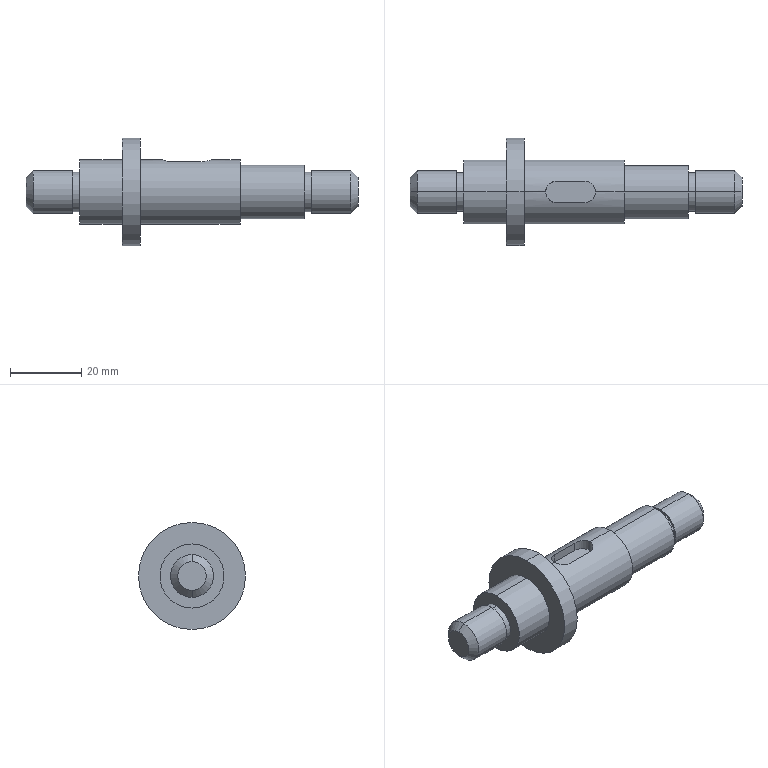Part | NX | features BREP 1 | 1 solid | 35 faces | box 93 x 30 x 30 mm | volume 19864 mm3 | cylinder 19 | plane 12 | cone 4 | commonest cylinder face diameters 11 x4 12 x4 18 x4 6 x3 15 x2 30 x2
STEP:
#1=CARTESIAN_POINT('',(11.521,0.,6.));
#2=VERTEX_POINT('',#1);
#3=CARTESIAN_POINT('',(8.521,3.,6.));
#4=VERTEX_POINT('',#3);
#5=CARTESIAN_POINT('',(8.521,0.,6.));
#6=DIRECTION('',(0.,0.,1.));
#7=DIRECTION('',(1.,0.,0.));
#8=AXIS2_PLACEMENT_3D('',#5,#6,#7);
#9=CIRCLE('',#8,3.);
#10=EDGE_CURVE('',#2,#4,#9,.T.);
#11=ORIENTED_EDGE('',*,*,#10,.F.);
#12=CARTESIAN_POINT('',(11.521,0.,9.));
#13=VERTEX_POINT('',#12);
#14=CARTESIAN_POINT('',(11.521,0.,6.));
#15=DIRECTION('',(0.,0.,1.));
#16=VECTOR('',#15,1000.);
#17=LINE('',#14,#16);
#18=EDGE_CURVE('',#2,#13,#17,.T.);
#19=ORIENTED_EDGE('',*,*,#18,.T.);
#20=CARTESIAN_POINT('',(8.521,3.,8.485));
#21=VERTEX_POINT('',#20);
#22=CARTESIAN_POINT('',(8.521,3.,8.485));
#23=CARTESIAN_POINT('',(9.32,3.,8.485));
#24=CARTESIAN_POINT('',(10.863,2.345,8.75));
#25=CARTESIAN_POINT('',(11.521,0.7985,9.));
#26=CARTESIAN_POINT('',(11.521,0.,9.));
#27=B_SPLINE_CURVE_WITH_KNOTS('',3,(#22,#23,#24,#25,#26),.UNSPECIFIED.,.F.,.F.,(4,1,4),(0.,0.00236,0.004721),.UNSPECIFIED.);
#28=EDGE_CURVE('',#21,#13,#27,.T.);
#29=ORIENTED_EDGE('',*,*,#28,.F.);
#30=CARTESIAN_POINT('',(8.521,3.,6.));
#31=DIRECTION('',(0.,0.,1.));
#32=VECTOR('',#31,1000.);
#33=LINE('',#30,#32);
#34=EDGE_CURVE('',#4,#21,#33,.T.);
#35=ORIENTED_EDGE('',*,*,#34,.F.);
#36=EDGE_LOOP('',(#11,#19,#29,#35));
#37=FACE_BOUND('',#36,.T.);
#38=CARTESIAN_POINT('',(8.521,0.,6.));
#39=DIRECTION('',(0.,0.,1.));
#40=DIRECTION('',(-1.,0.,0.));
#41=AXIS2_PLACEMENT_3D('',#38,#39,#40);
#42=CYLINDRICAL_SURFACE('',#41,3.);
#43=ADVANCED_FACE('',(#37),#42,.F.);
#44=CARTESIAN_POINT('',(52.521,0.,4.));
#45=VERTEX_POINT('',#44);
#46=CARTESIAN_POINT('',(52.521,0.,-4.));
#47=VERTEX_POINT('',#46);
#48=CARTESIAN_POINT('',(52.521,0.,0.));
#49=DIRECTION('',(-1.,0.,0.));
#50=DIRECTION('',(0.,0.,1.));
#51=AXIS2_PLACEMENT_3D('',#48,#49,#50);
#52=CIRCLE('',#51,4.);
#53=EDGE_CURVE('',#45,#47,#52,.T.);
#54=ORIENTED_EDGE('',*,*,#53,.T.);
#55=CARTESIAN_POINT('',(50.521,0.,-6.));
#56=VERTEX_POINT('',#55);
#57=CARTESIAN_POINT('',(52.521,0.,-4.));
#58=DIRECTION('',(-0.7071,0.,-0.7071));
#59=VECTOR('',#58,1000.);
#60=LINE('',#57,#59);
#61=EDGE_CURVE('',#47,#56,#60,.T.);
#62=ORIENTED_EDGE('',*,*,#61,.T.);
#63=CARTESIAN_POINT('',(50.521,0.,6.));
#64=VERTEX_POINT('',#63);
#65=CARTESIAN_POINT('',(50.521,0.,0.));
#66=DIRECTION('',(-1.,0.,0.));
#67=DIRECTION('',(0.,0.,1.));
#68=AXIS2_PLACEMENT_3D('',#65,#66,#67);
#69=CIRCLE('',#68,6.);
#70=EDGE_CURVE('',#64,#56,#69,.T.);
#71=ORIENTED_EDGE('',*,*,#70,.F.);
#72=CARTESIAN_POINT('',(52.521,0.,4.));
#73=DIRECTION('',(-0.7071,0.,0.7071));
#74=VECTOR('',#73,1000.);
#75=LINE('',#72,#74);
#76=EDGE_CURVE('',#45,#64,#75,.T.);
#77=ORIENTED_EDGE('',*,*,#76,.F.);
#78=EDGE_LOOP('',(#54,#62,#71,#77));
#79=FACE_BOUND('',#78,.T.);
#80=CARTESIAN_POINT('',(52.521,0.,0.));
#81=DIRECTION('',(-1.,0.,0.));
#82=DIRECTION('',(0.,0.,-1.));
#83=AXIS2_PLACEMENT_3D('',#80,#81,#82);
#84=CONICAL_SURFACE('',#83,4.,0.7854);
#85=ADVANCED_FACE('',(#79),#84,.T.);
#86=ORIENTED_EDGE('',*,*,#70,.T.);
#87=CARTESIAN_POINT('',(39.521,0.,-6.));
#88=VERTEX_POINT('',#87);
#89=CARTESIAN_POINT('',(-58.998,0.,-6.));
#90=DIRECTION('',(-1.,0.,0.));
#91=VECTOR('',#90,1000.);
#92=LINE('',#89,#91);
#93=EDGE_CURVE('',#56,#88,#92,.T.);
#94=ORIENTED_EDGE('',*,*,#93,.T.);
#95=CARTESIAN_POINT('',(39.521,0.,6.));
#96=VERTEX_POINT('',#95);
#97=CARTESIAN_POINT('',(39.521,0.,0.));
#98=DIRECTION('',(-1.,0.,0.));
#99=DIRECTION('',(0.,0.,1.));
#100=AXIS2_PLACEMENT_3D('',#97,#98,#99);
#101=CIRCLE('',#100,6.);
#102=EDGE_CURVE('',#96,#88,#101,.T.);
#103=ORIENTED_EDGE('',*,*,#102,.F.);
#104=CARTESIAN_POINT('',(-58.998,0.,6.));
#105=DIRECTION('',(-1.,0.,0.));
#106=VECTOR('',#105,1000.);
#107=LINE('',#104,#106);
#108=EDGE_CURVE('',#64,#96,#107,.T.);
#109=ORIENTED_EDGE('',*,*,#108,.F.);
#110=EDGE_LOOP('',(#86,#94,#103,#109));
#111=FACE_BOUND('',#110,.T.);
#112=CARTESIAN_POINT('',(-58.998,0.,0.));
#113=DIRECTION('',(-1.,0.,0.));
#114=DIRECTION('',(0.,0.,-1.));
#115=AXIS2_PLACEMENT_3D('',#112,#113,#114);
#116=CYLINDRICAL_SURFACE('',#115,6.);
#117=ADVANCED_FACE('',(#111),#116,.T.);
#118=CARTESIAN_POINT('',(39.521,0.,5.5));
#119=VERTEX_POINT('',#118);
#120=CARTESIAN_POINT('',(39.521,0.,-5.5));
#121=VERTEX_POINT('',#120);
#122=CARTESIAN_POINT('',(39.521,0.,0.));
#123=DIRECTION('',(-1.,0.,0.));
#124=DIRECTION('',(0.,0.,1.));
#125=AXIS2_PLACEMENT_3D('',#122,#123,#124);
#126=CIRCLE('',#125,5.5);
#127=EDGE_CURVE('',#119,#121,#126,.T.);
#128=ORIENTED_EDGE('',*,*,#127,.T.);
#129=CARTESIAN_POINT('',(37.521,0.,-5.5));
#130=VERTEX_POINT('',#129);
#131=CARTESIAN_POINT('',(-58.998,0.,-5.5));
#132=DIRECTION('',(-1.,0.,0.));
#133=VECTOR('',#132,1000.);
#134=LINE('',#131,#133);
#135=EDGE_CURVE('',#121,#130,#134,.T.);
#136=ORIENTED_EDGE('',*,*,#135,.T.);
#137=CARTESIAN_POINT('',(37.521,0.,5.5));
#138=VERTEX_POINT('',#137);
#139=CARTESIAN_POINT('',(37.521,0.,0.));
#140=DIRECTION('',(-1.,0.,0.));
#141=DIRECTION('',(0.,0.,1.));
#142=AXIS2_PLACEMENT_3D('',#139,#140,#141);
#143=CIRCLE('',#142,5.5);
#144=EDGE_CURVE('',#138,#130,#143,.T.);
#145=ORIENTED_EDGE('',*,*,#144,.F.);
#146=CARTESIAN_POINT('',(-58.998,0.,5.5));
#147=DIRECTION('',(-1.,0.,0.));
#148=VECTOR('',#147,1000.);
#149=LINE('',#146,#148);
#150=EDGE_CURVE('',#119,#138,#149,.T.);
#151=ORIENTED_EDGE('',*,*,#150,.F.);
#152=EDGE_LOOP('',(#128,#136,#145,#151));
#153=FACE_BOUND('',#152,.T.);
#154=CARTESIAN_POINT('',(-58.998,0.,0.));
#155=DIRECTION('',(-1.,0.,0.));
#156=DIRECTION('',(0.,0.,-1.));
#157=AXIS2_PLACEMENT_3D('',#154,#155,#156);
#158=CYLINDRICAL_SURFACE('',#157,5.5);
#159=ADVANCED_FACE('',(#153),#158,.T.);
#160=CARTESIAN_POINT('',(37.521,0.,7.5));
#161=VERTEX_POINT('',#160);
#162=CARTESIAN_POINT('',(37.521,0.,-7.5));
#163=VERTEX_POINT('',#162);
#164=CARTESIAN_POINT('',(37.521,0.,0.));
#165=DIRECTION('',(-1.,0.,0.));
#166=DIRECTION('',(0.,0.,1.));
#167=AXIS2_PLACEMENT_3D('',#164,#165,#166);
#168=CIRCLE('',#167,7.5);
#169=EDGE_CURVE('',#161,#163,#168,.T.);
#170=ORIENTED_EDGE('',*,*,#169,.T.);
#171=CARTESIAN_POINT('',(19.521,0.,-7.5));
#172=VERTEX_POINT('',#171);
#173=CARTESIAN_POINT('',(-58.998,0.,-7.5));
#174=DIRECTION('',(-1.,0.,0.));
#175=VECTOR('',#174,1000.);
#176=LINE('',#173,#175);
#177=EDGE_CURVE('',#163,#172,#176,.T.);
#178=ORIENTED_EDGE('',*,*,#177,.T.);
#179=CARTESIAN_POINT('',(19.521,0.,7.5));
#180=VERTEX_POINT('',#179);
#181=CARTESIAN_POINT('',(19.521,0.,0.));
#182=DIRECTION('',(-1.,0.,0.));
#183=DIRECTION('',(0.,0.,1.));
#184=AXIS2_PLACEMENT_3D('',#181,#182,#183);
#185=CIRCLE('',#184,7.5);
#186=EDGE_CURVE('',#180,#172,#185,.T.);
#187=ORIENTED_EDGE('',*,*,#186,.F.);
#188=CARTESIAN_POINT('',(-58.998,0.,7.5));
#189=DIRECTION('',(-1.,0.,0.));
#190=VECTOR('',#189,1000.);
#191=LINE('',#188,#190);
#192=EDGE_CURVE('',#161,#180,#191,.T.);
#193=ORIENTED_EDGE('',*,*,#192,.F.);
#194=EDGE_LOOP('',(#170,#178,#187,#193));
#195=FACE_BOUND('',#194,.T.);
#196=CARTESIAN_POINT('',(-58.998,0.,0.));
#197=DIRECTION('',(-1.,0.,0.));
#198=DIRECTION('',(0.,0.,-1.));
#199=AXIS2_PLACEMENT_3D('',#196,#197,#198);
#200=CYLINDRICAL_SURFACE('',#199,7.5);
#201=ADVANCED_FACE('',(#195),#200,.T.);
#202=CARTESIAN_POINT('',(19.521,0.,9.));
#203=VERTEX_POINT('',#202);
#204=CARTESIAN_POINT('',(19.521,0.,-9.));
#205=VERTEX_POINT('',#204);
#206=CARTESIAN_POINT('',(19.521,0.,0.));
#207=DIRECTION('',(-1.,0.,0.));
#208=DIRECTION('',(0.,0.,1.));
#209=AXIS2_PLACEMENT_3D('',#206,#207,#208);
#210=CIRCLE('',#209,9.);
#211=EDGE_CURVE('',#203,#205,#210,.T.);
#212=ORIENTED_EDGE('',*,*,#211,.T.);
#213=CARTESIAN_POINT('',(-8.479,0.,-9.));
#214=VERTEX_POINT('',#213);
#215=CARTESIAN_POINT('',(-58.998,0.,-9.));
#216=DIRECTION('',(-1.,0.,0.));
#217=VECTOR('',#216,1000.);
#218=LINE('',#215,#217);
#219=EDGE_CURVE('',#205,#214,#218,.T.);
#220=ORIENTED_EDGE('',*,*,#219,.T.);
#221=CARTESIAN_POINT('',(-8.479,0.,9.));
#222=VERTEX_POINT('',#221);
#223=CARTESIAN_POINT('',(-8.479,0.,0.));
#224=DIRECTION('',(-1.,0.,0.));
#225=DIRECTION('',(0.,0.,1.));
#226=AXIS2_PLACEMENT_3D('',#223,#224,#225);
#227=CIRCLE('',#226,9.);
#228=EDGE_CURVE('',#222,#214,#227,.T.);
#229=ORIENTED_EDGE('',*,*,#228,.F.);
#230=CARTESIAN_POINT('',(-2.479,0.,9.));
#231=VERTEX_POINT('',#230);
#232=CARTESIAN_POINT('',(-58.998,0.,9.));
#233=DIRECTION('',(-1.,0.,0.));
#234=VECTOR('',#233,1000.);
#235=LINE('',#232,#234);
#236=EDGE_CURVE('',#231,#222,#235,.T.);
#237=ORIENTED_EDGE('',*,*,#236,.F.);
#238=CARTESIAN_POINT('',(0.5211,3.,8.485));
#239=VERTEX_POINT('',#238);
#240=CARTESIAN_POINT('',(-2.479,0.,9.));
#241=CARTESIAN_POINT('',(-2.479,0.7985,9.));
#242=CARTESIAN_POINT('',(-1.822,2.343,8.75));
#243=CARTESIAN_POINT('',(-0.2774,3.,8.485));
#244=CARTESIAN_POINT('',(0.5211,3.,8.485));
#245=B_SPLINE_CURVE_WITH_KNOTS('',3,(#240,#241,#242,#243,#244),.UNSPECIFIED.,.F.,.F.,(4,1,4),(0.,0.00236,0.004721),.UNSPECIFIED.);
#246=EDGE_CURVE('',#231,#239,#245,.T.);
#247=ORIENTED_EDGE('',*,*,#246,.T.);
#248=CARTESIAN_POINT('',(-58.998,3.,8.485));
#249=DIRECTION('',(1.,0.,0.));
#250=VECTOR('',#249,1000.);
#251=LINE('',#248,#250);
#252=EDGE_CURVE('',#239,#21,#251,.T.);
#253=ORIENTED_EDGE('',*,*,#252,.T.);
#254=ORIENTED_EDGE('',*,*,#28,.T.);
#255=CARTESIAN_POINT('',(-58.998,0.,9.));
#256=DIRECTION('',(-1.,0.,0.));
#257=VECTOR('',#256,1000.);
#258=LINE('',#255,#257);
#259=EDGE_CURVE('',#203,#13,#258,.T.);
#260=ORIENTED_EDGE('',*,*,#259,.F.);
#261=EDGE_LOOP('',(#212,#220,#229,#237,#247,#253,#254,#260));
#262=FACE_BOUND('',#261,.T.);
#263=CARTESIAN_POINT('',(-58.998,0.,0.));
#264=DIRECTION('',(-1.,0.,0.));
#265=DIRECTION('',(0.,0.,-1.));
#266=AXIS2_PLACEMENT_3D('',#263,#264,#265);
#267=CYLINDRICAL_SURFACE('',#266,9.);
#268=ADVANCED_FACE('',(#262),#267,.T.);
#269=CARTESIAN_POINT('',(-8.479,0.,15.));
#270=VERTEX_POINT('',#269);
#271=CARTESIAN_POINT('',(-8.479,0.,-15.));
#272=VERTEX_POINT('',#271);
#273=CARTESIAN_POINT('',(-8.479,0.,0.));
#274=DIRECTION('',(-1.,0.,0.));
#275=DIRECTION('',(0.,0.,1.));
#276=AXIS2_PLACEMENT_3D('',#273,#274,#275);
#277=CIRCLE('',#276,15.);
#278=EDGE_CURVE('',#270,#272,#277,.T.);
#279=ORIENTED_EDGE('',*,*,#278,.T.);
#280=CARTESIAN_POINT('',(-13.479,0.,-15.));
#281=VERTEX_POINT('',#280);
#282=CARTESIAN_POINT('',(-58.998,0.,-15.));
#283=DIRECTION('',(-1.,0.,0.));
#284=VECTOR('',#283,1000.);
#285=LINE('',#282,#284);
#286=EDGE_CURVE('',#272,#281,#285,.T.);
#287=ORIENTED_EDGE('',*,*,#286,.T.);
#288=CARTESIAN_POINT('',(-13.479,0.,15.));
#289=VERTEX_POINT('',#288);
#290=CARTESIAN_POINT('',(-13.479,0.,0.));
#291=DIRECTION('',(-1.,0.,0.));
#292=DIRECTION('',(0.,0.,1.));
#293=AXIS2_PLACEMENT_3D('',#290,#291,#292);
#294=CIRCLE('',#293,15.);
#295=EDGE_CURVE('',#289,#281,#294,.T.);
#296=ORIENTED_EDGE('',*,*,#295,.F.);
#297=CARTESIAN_POINT('',(-58.998,0.,15.));
#298=DIRECTION('',(-1.,0.,0.));
#299=VECTOR('',#298,1000.);
#300=LINE('',#297,#299);
#301=EDGE_CURVE('',#270,#289,#300,.T.);
#302=ORIENTED_EDGE('',*,*,#301,.F.);
#303=EDGE_LOOP('',(#279,#287,#296,#302));
#304=FACE_BOUND('',#303,.T.);
#305=CARTESIAN_POINT('',(-58.998,0.,0.));
#306=DIRECTION('',(-1.,0.,0.));
#307=DIRECTION('',(0.,0.,-1.));
#308=AXIS2_PLACEMENT_3D('',#305,#306,#307);
#309=CYLINDRICAL_SURFACE('',#308,15.);
#310=ADVANCED_FACE('',(#304),#309,.T.);
#311=CARTESIAN_POINT('',(-13.479,0.,9.));
#312=VERTEX_POINT('',#311);
#313=CARTESIAN_POINT('',(-13.479,0.,-9.));
#314=VERTEX_POINT('',#313);
#315=CARTESIAN_POINT('',(-13.479,0.,0.));
#316=DIRECTION('',(-1.,0.,0.));
#317=DIRECTION('',(0.,0.,1.));
#318=AXIS2_PLACEMENT_3D('',#315,#316,#317);
#319=CIRCLE('',#318,9.);
#320=EDGE_CURVE('',#312,#314,#319,.T.);
#321=ORIENTED_EDGE('',*,*,#320,.T.);
#322=CARTESIAN_POINT('',(-25.479,0.,-9.));
#323=VERTEX_POINT('',#322);
#324=CARTESIAN_POINT('',(-58.998,0.,-9.));
#325=DIRECTION('',(-1.,0.,0.));
#326=VECTOR('',#325,1000.);
#327=LINE('',#324,#326);
#328=EDGE_CURVE('',#314,#323,#327,.T.);
#329=ORIENTED_EDGE('',*,*,#328,.T.);
#330=CARTESIAN_POINT('',(-25.479,0.,9.));
#331=VERTEX_POINT('',#330);
#332=CARTESIAN_POINT('',(-25.479,0.,0.));
#333=DIRECTION('',(-1.,0.,0.));
#334=DIRECTION('',(0.,0.,1.));
#335=AXIS2_PLACEMENT_3D('',#332,#333,#334);
#336=CIRCLE('',#335,9.);
#337=EDGE_CURVE('',#331,#323,#336,.T.);
#338=ORIENTED_EDGE('',*,*,#337,.F.);
#339=CARTESIAN_POINT('',(-58.998,0.,9.));
#340=DIRECTION('',(-1.,0.,0.));
#341=VECTOR('',#340,1000.);
#342=LINE('',#339,#341);
#343=EDGE_CURVE('',#312,#331,#342,.T.);
#344=ORIENTED_EDGE('',*,*,#343,.F.);
#345=EDGE_LOOP('',(#321,#329,#338,#344));
#346=FACE_BOUND('',#345,.T.);
#347=CARTESIAN_POINT('',(-58.998,0.,0.));
#348=DIRECTION('',(-1.,0.,0.));
#349=DIRECTION('',(0.,0.,-1.));
#350=AXIS2_PLACEMENT_3D('',#347,#348,#349);
#351=CYLINDRICAL_SURFACE('',#350,9.);
#352=ADVANCED_FACE('',(#346),#351,.T.);
#353=CARTESIAN_POINT('',(-25.479,0.,5.5));
#354=VERTEX_POINT('',#353);
#355=CARTESIAN_POINT('',(-25.479,0.,-5.5));
#356=VERTEX_POINT('',#355);
#357=CARTESIAN_POINT('',(-25.479,0.,0.));
#358=DIRECTION('',(-1.,0.,0.));
#359=DIRECTION('',(0.,0.,1.));
#360=AXIS2_PLACEMENT_3D('',#357,#358,#359);
#361=CIRCLE('',#360,5.5);
#362=EDGE_CURVE('',#354,#356,#361,.T.);
#363=ORIENTED_EDGE('',*,*,#362,.T.);
#364=CARTESIAN_POINT('',(-27.479,0.,-5.5));
#365=VERTEX_POINT('',#364);
#366=CARTESIAN_POINT('',(-58.998,0.,-5.5));
#367=DIRECTION('',(-1.,0.,0.));
#368=VECTOR('',#367,1000.);
#369=LINE('',#366,#368);
#370=EDGE_CURVE('',#356,#365,#369,.T.);
#371=ORIENTED_EDGE('',*,*,#370,.T.);
#372=CARTESIAN_POINT('',(-27.479,0.,5.5));
#373=VERTEX_POINT('',#372);
#374=CARTESIAN_POINT('',(-27.479,0.,0.));
#375=DIRECTION('',(-1.,0.,0.));
#376=DIRECTION('',(0.,0.,1.));
#377=AXIS2_PLACEMENT_3D('',#374,#375,#376);
#378=CIRCLE('',#377,5.5);
#379=EDGE_CURVE('',#373,#365,#378,.T.);
#380=ORIENTED_EDGE('',*,*,#379,.F.);
#381=CARTESIAN_POINT('',(-58.998,0.,5.5));
#382=DIRECTION('',(-1.,0.,0.));
#383=VECTOR('',#382,1000.);
#384=LINE('',#381,#383);
#385=EDGE_CURVE('',#354,#373,#384,.T.);
#386=ORIENTED_EDGE('',*,*,#385,.F.);
#387=EDGE_LOOP('',(#363,#371,#380,#386));
#388=FACE_BOUND('',#387,.T.);
#389=CARTESIAN_POINT('',(-58.998,0.,0.));
#390=DIRECTION('',(-1.,0.,0.));
#391=DIRECTION('',(0.,0.,-1.));
#392=AXIS2_PLACEMENT_3D('',#389,#390,#391);
#393=CYLINDRICAL_SURFACE('',#392,5.5);
#394=ADVANCED_FACE('',(#388),#393,.T.);
#395=CARTESIAN_POINT('',(-27.479,0.,6.));
#396=VERTEX_POINT('',#395);
#397=CARTESIAN_POINT('',(-27.479,0.,-6.));
#398=VERTEX_POINT('',#397);
#399=CARTESIAN_POINT('',(-27.479,0.,0.));
#400=DIRECTION('',(-1.,0.,0.));
#401=DIRECTION('',(0.,0.,1.));
#402=AXIS2_PLACEMENT_3D('',#399,#400,#401);
#403=CIRCLE('',#402,6.);
#404=EDGE_CURVE('',#396,#398,#403,.T.);
#405=ORIENTED_EDGE('',*,*,#404,.T.);
#406=CARTESIAN_POINT('',(-38.479,0.,-6.));
#407=VERTEX_POINT('',#406);
#408=CARTESIAN_POINT('',(-58.998,0.,-6.));
#409=DIRECTION('',(-1.,0.,0.));
#410=VECTOR('',#409,1000.);
#411=LINE('',#408,#410);
#412=EDGE_CURVE('',#398,#407,#411,.T.);
#413=ORIENTED_EDGE('',*,*,#412,.T.);
#414=CARTESIAN_POINT('',(-38.479,0.,6.));
#415=VERTEX_POINT('',#414);
#416=CARTESIAN_POINT('',(-38.479,0.,0.));
#417=DIRECTION('',(-1.,0.,0.));
#418=DIRECTION('',(0.,0.,1.));
#419=AXIS2_PLACEMENT_3D('',#416,#417,#418);
#420=CIRCLE('',#419,6.);
#421=EDGE_CURVE('',#415,#407,#420,.T.);
#422=ORIENTED_EDGE('',*,*,#421,.F.);
#423=CARTESIAN_POINT('',(-58.998,0.,6.));
#424=DIRECTION('',(-1.,0.,0.));
#425=VECTOR('',#424,1000.);
#426=LINE('',#423,#425);
#427=EDGE_CURVE('',#396,#415,#426,.T.);
#428=ORIENTED_EDGE('',*,*,#427,.F.);
#429=EDGE_LOOP('',(#405,#413,#422,#428));
#430=FACE_BOUND('',#429,.T.);
#431=CARTESIAN_POINT('',(-58.998,0.,0.));
#432=DIRECTION('',(-1.,0.,0.));
#433=DIRECTION('',(0.,0.,-1.));
#434=AXIS2_PLACEMENT_3D('',#431,#432,#433);
#435=CYLINDRICAL_SURFACE('',#434,6.);
#436=ADVANCED_FACE('',(#430),#435,.T.);
#437=CARTESIAN_POINT('',(-40.479,0.,4.));
#438=VERTEX_POINT('',#437);
#439=CARTESIAN_POINT('',(-40.479,0.,-4.));
#440=VERTEX_POINT('',#439);
#441=CARTESIAN_POINT('',(-40.479,0.,0.));
#442=DIRECTION('',(-1.,0.,0.));
#443=DIRECTION('',(0.,0.,1.));
#444=AXIS2_PLACEMENT_3D('',#441,#442,#443);
#445=CIRCLE('',#444,4.);
#446=EDGE_CURVE('',#438,#440,#445,.T.);
#447=ORIENTED_EDGE('',*,*,#446,.F.);
#448=CARTESIAN_POINT('',(-38.479,0.,6.));
#449=DIRECTION('',(0.7071,0.,0.7071));
#450=VECTOR('',#449,1000.);
#451=LINE('',#448,#450);
#452=EDGE_CURVE('',#415,#438,#451,.F.);
#453=ORIENTED_EDGE('',*,*,#452,.F.);
#454=ORIENTED_EDGE('',*,*,#421,.T.);
#455=CARTESIAN_POINT('',(-38.479,0.,-6.));
#456=DIRECTION('',(0.7071,0.,-0.7071));
#457=VECTOR('',#456,1000.);
#458=LINE('',#455,#457);
#459=EDGE_CURVE('',#407,#440,#458,.F.);
#460=ORIENTED_EDGE('',*,*,#459,.T.);
#461=EDGE_LOOP('',(#447,#453,#454,#460));
#462=FACE_BOUND('',#461,.T.);
#463=CARTESIAN_POINT('',(-38.479,0.,0.));
#464=DIRECTION('',(1.,0.,0.));
#465=DIRECTION('',(0.,0.,1.));
#466=AXIS2_PLACEMENT_3D('',#463,#464,#465);
#467=CONICAL_SURFACE('',#466,6.,0.7854);
#468=ADVANCED_FACE('',(#462),#467,.T.);
#469=CARTESIAN_POINT('',(-40.479,0.,0.));
#470=DIRECTION('',(-1.,0.,0.));
#471=DIRECTION('',(0.,0.,1.));
#472=AXIS2_PLACEMENT_3D('',#469,#470,#471);
#473=CIRCLE('',#472,4.);
#474=EDGE_CURVE('',#440,#438,#473,.T.);
#475=ORIENTED_EDGE('',*,*,#474,.T.);
#476=ORIENTED_EDGE('',*,*,#446,.T.);
#477=EDGE_LOOP('',(#475,#476));
#478=FACE_BOUND('',#477,.T.);
#479=CARTESIAN_POINT('',(-40.479,0.,0.));
#480=DIRECTION('',(1.,0.,0.));
#481=DIRECTION('',(0.,1.,0.));
#482=AXIS2_PLACEMENT_3D('',#479,#480,#481);
#483=PLANE('',#482);
#484=ADVANCED_FACE('',(#478),#483,.F.);
#485=ORIENTED_EDGE('',*,*,#452,.T.);
#486=ORIENTED_EDGE('',*,*,#474,.F.);
#487=ORIENTED_EDGE('',*,*,#459,.F.);
#488=CARTESIAN_POINT('',(-38.479,0.,0.));
#489=DIRECTION('',(-1.,0.,0.));
#490=DIRECTION('',(0.,0.,1.));
#491=AXIS2_PLACEMENT_3D('',#488,#489,#490);
#492=CIRCLE('',#491,6.);
#493=EDGE_CURVE('',#407,#415,#492,.T.);
#494=ORIENTED_EDGE('',*,*,#493,.T.);
#495=EDGE_LOOP('',(#485,#486,#487,#494));
#496=FACE_BOUND('',#495,.T.);
#497=CARTESIAN_POINT('',(-38.479,0.,0.));
#498=DIRECTION('',(1.,0.,0.));
#499=DIRECTION('',(0.,0.,1.));
#500=AXIS2_PLACEMENT_3D('',#497,#498,#499);
#501=CONICAL_SURFACE('',#500,6.,0.7854);
#502=ADVANCED_FACE('',(#496),#501,.T.);
#503=ORIENTED_EDGE('',*,*,#412,.F.);
#504=CARTESIAN_POINT('',(-27.479,0.,0.));
#505=DIRECTION('',(-1.,0.,0.));
#506=DIRECTION('',(0.,0.,1.));
#507=AXIS2_PLACEMENT_3D('',#504,#505,#506);
#508=CIRCLE('',#507,6.);
#509=EDGE_CURVE('',#398,#396,#508,.T.);
#510=ORIENTED_EDGE('',*,*,#509,.T.);
#511=ORIENTED_EDGE('',*,*,#427,.T.);
#512=ORIENTED_EDGE('',*,*,#493,.F.);
#513=EDGE_LOOP('',(#503,#510,#511,#512));
#514=FACE_BOUND('',#513,.T.);
#515=CARTESIAN_POINT('',(-58.998,0.,0.));
#516=DIRECTION('',(-1.,0.,0.));
#517=DIRECTION('',(0.,0.,-1.));
#518=AXIS2_PLACEMENT_3D('',#515,#516,#517);
#519=CYLINDRICAL_SURFACE('',#518,6.);
#520=ADVANCED_FACE('',(#514),#519,.T.);
#521=ORIENTED_EDGE('',*,*,#404,.F.);
#522=ORIENTED_EDGE('',*,*,#509,.F.);
#523=EDGE_LOOP('',(#521,#522));
#524=FACE_BOUND('',#523,.T.);
#525=ORIENTED_EDGE('',*,*,#379,.T.);
#526=CARTESIAN_POINT('',(-27.479,0.,0.));
#527=DIRECTION('',(-1.,0.,0.));
#528=DIRECTION('',(0.,0.,1.));
#529=AXIS2_PLACEMENT_3D('',#526,#527,#528);
#530=CIRCLE('',#529,5.5);
#531=EDGE_CURVE('',#365,#373,#530,.T.);
#532=ORIENTED_EDGE('',*,*,#531,.T.);
#533=EDGE_LOOP('',(#525,#532));
#534=FACE_BOUND('',#533,.T.);
#535=CARTESIAN_POINT('',(-27.479,6.,0.));
#536=DIRECTION('',(-1.,0.,0.));
#537=DIRECTION('',(0.,0.,-1.));
#538=AXIS2_PLACEMENT_3D('',#535,#536,#537);
#539=PLANE('',#538);
#540=ADVANCED_FACE('',(#524,#534),#539,.F.);
#541=ORIENTED_EDGE('',*,*,#370,.F.);
#542=CARTESIAN_POINT('',(-25.479,0.,0.));
#543=DIRECTION('',(-1.,0.,0.));
#544=DIRECTION('',(0.,0.,1.));
#545=AXIS2_PLACEMENT_3D('',#542,#543,#544);
#546=CIRCLE('',#545,5.5);
#547=EDGE_CURVE('',#356,#354,#546,.T.);
#548=ORIENTED_EDGE('',*,*,#547,.T.);
#549=ORIENTED_EDGE('',*,*,#385,.T.);
#550=ORIENTED_EDGE('',*,*,#531,.F.);
#551=EDGE_LOOP('',(#541,#548,#549,#550));
#552=FACE_BOUND('',#551,.T.);
#553=CARTESIAN_POINT('',(-58.998,0.,0.));
#554=DIRECTION('',(-1.,0.,0.));
#555=DIRECTION('',(0.,0.,-1.));
#556=AXIS2_PLACEMENT_3D('',#553,#554,#555);
#557=CYLINDRICAL_SURFACE('',#556,5.5);
#558=ADVANCED_FACE('',(#552),#557,.T.);
#559=ORIENTED_EDGE('',*,*,#337,.T.);
#560=CARTESIAN_POINT('',(-25.479,0.,0.));
#561=DIRECTION('',(-1.,0.,0.));
#562=DIRECTION('',(0.,0.,1.));
#563=AXIS2_PLACEMENT_3D('',#560,#561,#562);
#564=CIRCLE('',#563,9.);
#565=EDGE_CURVE('',#323,#331,#564,.T.);
#566=ORIENTED_EDGE('',*,*,#565,.T.);
#567=EDGE_LOOP('',(#559,#566));
#568=FACE_BOUND('',#567,.T.);
#569=ORIENTED_EDGE('',*,*,#362,.F.);
#570=ORIENTED_EDGE('',*,*,#547,.F.);
#571=EDGE_LOOP('',(#569,#570));
#572=FACE_BOUND('',#571,.T.);
#573=CARTESIAN_POINT('',(-25.479,5.5,0.));
#574=DIRECTION('',(1.,0.,0.));
#575=DIRECTION('',(0.,1.,0.));
#576=AXIS2_PLACEMENT_3D('',#573,#574,#575);
#577=PLANE('',#576);
#578=ADVANCED_FACE('',(#568,#572),#577,.F.);
#579=ORIENTED_EDGE('',*,*,#328,.F.);
#580=CARTESIAN_POINT('',(-13.479,0.,0.));
#581=DIRECTION('',(-1.,0.,0.));
#582=DIRECTION('',(0.,0.,1.));
#583=AXIS2_PLACEMENT_3D('',#580,#581,#582);
#584=CIRCLE('',#583,9.);
#585=EDGE_CURVE('',#314,#312,#584,.T.);
#586=ORIENTED_EDGE('',*,*,#585,.T.);
#587=ORIENTED_EDGE('',*,*,#343,.T.);
#588=ORIENTED_EDGE('',*,*,#565,.F.);
#589=EDGE_LOOP('',(#579,#586,#587,#588));
#590=FACE_BOUND('',#589,.T.);
#591=CARTESIAN_POINT('',(-58.998,0.,0.));
#592=DIRECTION('',(-1.,0.,0.));
#593=DIRECTION('',(0.,0.,-1.));
#594=AXIS2_PLACEMENT_3D('',#591,#592,#593);
#595=CYLINDRICAL_SURFACE('',#594,9.);
#596=ADVANCED_FACE('',(#590),#595,.T.);
#597=ORIENTED_EDGE('',*,*,#295,.T.);
#598=CARTESIAN_POINT('',(-13.479,0.,0.));
#599=DIRECTION('',(-1.,0.,0.));
#600=DIRECTION('',(0.,0.,1.));
#601=AXIS2_PLACEMENT_3D('',#598,#599,#600);
#602=CIRCLE('',#601,15.);
#603=EDGE_CURVE('',#281,#289,#602,.T.);
#604=ORIENTED_EDGE('',*,*,#603,.T.);
#605=EDGE_LOOP('',(#597,#604));
#606=FACE_BOUND('',#605,.T.);
#607=ORIENTED_EDGE('',*,*,#320,.F.);
#608=ORIENTED_EDGE('',*,*,#585,.F.);
#609=EDGE_LOOP('',(#607,#608));
#610=FACE_BOUND('',#609,.T.);
#611=CARTESIAN_POINT('',(-13.479,9.,0.));
#612=DIRECTION('',(1.,0.,0.));
#613=DIRECTION('',(0.,1.,0.));
#614=AXIS2_PLACEMENT_3D('',#611,#612,#613);
#615=PLANE('',#614);
#616=ADVANCED_FACE('',(#606,#610),#615,.F.);
#617=ORIENTED_EDGE('',*,*,#286,.F.);
#618=CARTESIAN_POINT('',(-8.479,0.,0.));
#619=DIRECTION('',(-1.,0.,0.));
#620=DIRECTION('',(0.,0.,1.));
#621=AXIS2_PLACEMENT_3D('',#618,#619,#620);
#622=CIRCLE('',#621,15.);
#623=EDGE_CURVE('',#272,#270,#622,.T.);
#624=ORIENTED_EDGE('',*,*,#623,.T.);
#625=ORIENTED_EDGE('',*,*,#301,.T.);
#626=ORIENTED_EDGE('',*,*,#603,.F.);
#627=EDGE_LOOP('',(#617,#624,#625,#626));
#628=FACE_BOUND('',#627,.T.);
#629=CARTESIAN_POINT('',(-58.998,0.,0.));
#630=DIRECTION('',(-1.,0.,0.));
#631=DIRECTION('',(0.,0.,-1.));
#632=AXIS2_PLACEMENT_3D('',#629,#630,#631);
#633=CYLINDRICAL_SURFACE('',#632,15.);
#634=ADVANCED_FACE('',(#628),#633,.T.);
#635=ORIENTED_EDGE('',*,*,#278,.F.);
#636=ORIENTED_EDGE('',*,*,#623,.F.);
#637=EDGE_LOOP('',(#635,#636));
#638=FACE_BOUND('',#637,.T.);
#639=ORIENTED_EDGE('',*,*,#228,.T.);
#640=CARTESIAN_POINT('',(-8.479,0.,0.));
#641=DIRECTION('',(-1.,0.,0.));
#642=DIRECTION('',(0.,0.,1.));
#643=AXIS2_PLACEMENT_3D('',#640,#641,#642);
#644=CIRCLE('',#643,9.);
#645=EDGE_CURVE('',#214,#222,#644,.T.);
#646=ORIENTED_EDGE('',*,*,#645,.T.);
#647=EDGE_LOOP('',(#639,#646));
#648=FACE_BOUND('',#647,.T.);
#649=CARTESIAN_POINT('',(-8.479,15.,0.));
#650=DIRECTION('',(-1.,0.,0.));
#651=DIRECTION('',(0.,0.,-1.));
#652=AXIS2_PLACEMENT_3D('',#649,#650,#651);
#653=PLANE('',#652);
#654=ADVANCED_FACE('',(#638,#648),#653,.F.);
#655=ORIENTED_EDGE('',*,*,#219,.F.);
#656=CARTESIAN_POINT('',(19.521,0.,0.));
#657=DIRECTION('',(-1.,0.,0.));
#658=DIRECTION('',(0.,0.,1.));
#659=AXIS2_PLACEMENT_3D('',#656,#657,#658);
#660=CIRCLE('',#659,9.);
#661=EDGE_CURVE('',#205,#203,#660,.T.);
#662=ORIENTED_EDGE('',*,*,#661,.T.);
#663=ORIENTED_EDGE('',*,*,#259,.T.);
#664=CARTESIAN_POINT('',(8.521,-3.,8.485));
#665=VERTEX_POINT('',#664);
#666=CARTESIAN_POINT('',(11.521,0.,9.));
#667=CARTESIAN_POINT('',(11.521,-0.7985,9.));
#668=CARTESIAN_POINT('',(10.865,-2.343,8.75));
#669=CARTESIAN_POINT('',(9.32,-3.,8.485));
#670=CARTESIAN_POINT('',(8.521,-3.,8.485));
#671=B_SPLINE_CURVE_WITH_KNOTS('',3,(#666,#667,#668,#669,#670),.UNSPECIFIED.,.F.,.F.,(4,1,4),(0.,0.00236,0.004721),.UNSPECIFIED.);
#672=EDGE_CURVE('',#13,#665,#671,.T.);
#673=ORIENTED_EDGE('',*,*,#672,.T.);
#674=CARTESIAN_POINT('',(0.5211,-3.,8.485));
#675=VERTEX_POINT('',#674);
#676=CARTESIAN_POINT('',(-58.998,-3.,8.485));
#677=DIRECTION('',(-1.,0.,0.));
#678=VECTOR('',#677,1000.);
#679=LINE('',#676,#678);
#680=EDGE_CURVE('',#665,#675,#679,.T.);
#681=ORIENTED_EDGE('',*,*,#680,.T.);
#682=CARTESIAN_POINT('',(0.5211,-3.,8.485));
#683=CARTESIAN_POINT('',(-0.2774,-3.,8.485));
#684=CARTESIAN_POINT('',(-1.821,-2.345,8.75));
#685=CARTESIAN_POINT('',(-2.479,-0.7985,9.));
#686=CARTESIAN_POINT('',(-2.479,0.,9.));
#687=B_SPLINE_CURVE_WITH_KNOTS('',3,(#682,#683,#684,#685,#686),.UNSPECIFIED.,.F.,.F.,(4,1,4),(0.,0.00236,0.004721),.UNSPECIFIED.);
#688=EDGE_CURVE('',#675,#231,#687,.T.);
#689=ORIENTED_EDGE('',*,*,#688,.T.);
#690=ORIENTED_EDGE('',*,*,#236,.T.);
#691=ORIENTED_EDGE('',*,*,#645,.F.);
#692=EDGE_LOOP('',(#655,#662,#663,#673,#681,#689,#690,#691));
#693=FACE_BOUND('',#692,.T.);
#694=CARTESIAN_POINT('',(-58.998,0.,0.));
#695=DIRECTION('',(-1.,0.,0.));
#696=DIRECTION('',(0.,0.,-1.));
#697=AXIS2_PLACEMENT_3D('',#694,#695,#696);
#698=CYLINDRICAL_SURFACE('',#697,9.);
#699=ADVANCED_FACE('',(#693),#698,.T.);
#700=ORIENTED_EDGE('',*,*,#211,.F.);
#701=ORIENTED_EDGE('',*,*,#661,.F.);
#702=EDGE_LOOP('',(#700,#701));
#703=FACE_BOUND('',#702,.T.);
#704=ORIENTED_EDGE('',*,*,#186,.T.);
#705=CARTESIAN_POINT('',(19.521,0.,0.));
#706=DIRECTION('',(-1.,0.,0.));
#707=DIRECTION('',(0.,0.,1.));
#708=AXIS2_PLACEMENT_3D('',#705,#706,#707);
#709=CIRCLE('',#708,7.5);
#710=EDGE_CURVE('',#172,#180,#709,.T.);
#711=ORIENTED_EDGE('',*,*,#710,.T.);
#712=EDGE_LOOP('',(#704,#711));
#713=FACE_BOUND('',#712,.T.);
#714=CARTESIAN_POINT('',(19.521,9.,0.));
#715=DIRECTION('',(-1.,0.,0.));
#716=DIRECTION('',(0.,0.,-1.));
#717=AXIS2_PLACEMENT_3D('',#714,#715,#716);
#718=PLANE('',#717);
#719=ADVANCED_FACE('',(#703,#713),#718,.F.);
#720=ORIENTED_EDGE('',*,*,#177,.F.);
#721=CARTESIAN_POINT('',(37.521,0.,0.));
#722=DIRECTION('',(-1.,0.,0.));
#723=DIRECTION('',(0.,0.,1.));
#724=AXIS2_PLACEMENT_3D('',#721,#722,#723);
#725=CIRCLE('',#724,7.5);
#726=EDGE_CURVE('',#163,#161,#725,.T.);
#727=ORIENTED_EDGE('',*,*,#726,.T.);
#728=ORIENTED_EDGE('',*,*,#192,.T.);
#729=ORIENTED_EDGE('',*,*,#710,.F.);
#730=EDGE_LOOP('',(#720,#727,#728,#729));
#731=FACE_BOUND('',#730,.T.);
#732=CARTESIAN_POINT('',(-58.998,0.,0.));
#733=DIRECTION('',(-1.,0.,0.));
#734=DIRECTION('',(0.,0.,-1.));
#735=AXIS2_PLACEMENT_3D('',#732,#733,#734);
#736=CYLINDRICAL_SURFACE('',#735,7.5);
#737=ADVANCED_FACE('',(#731),#736,.T.);
#738=ORIENTED_EDGE('',*,*,#169,.F.);
#739=ORIENTED_EDGE('',*,*,#726,.F.);
#740=EDGE_LOOP('',(#738,#739));
#741=FACE_BOUND('',#740,.T.);
#742=ORIENTED_EDGE('',*,*,#144,.T.);
#743=CARTESIAN_POINT('',(37.521,0.,0.));
#744=DIRECTION('',(-1.,0.,0.));
#745=DIRECTION('',(0.,0.,1.));
#746=AXIS2_PLACEMENT_3D('',#743,#744,#745);
#747=CIRCLE('',#746,5.5);
#748=EDGE_CURVE('',#130,#138,#747,.T.);
#749=ORIENTED_EDGE('',*,*,#748,.T.);
#750=EDGE_LOOP('',(#742,#749));
#751=FACE_BOUND('',#750,.T.);
#752=CARTESIAN_POINT('',(37.521,7.5,0.));
#753=DIRECTION('',(-1.,0.,0.));
#754=DIRECTION('',(0.,0.,-1.));
#755=AXIS2_PLACEMENT_3D('',#752,#753,#754);
#756=PLANE('',#755);
#757=ADVANCED_FACE('',(#741,#751),#756,.F.);
#758=ORIENTED_EDGE('',*,*,#135,.F.);
#759=CARTESIAN_POINT('',(39.521,0.,0.));
#760=DIRECTION('',(-1.,0.,0.));
#761=DIRECTION('',(0.,0.,1.));
#762=AXIS2_PLACEMENT_3D('',#759,#760,#761);
#763=CIRCLE('',#762,5.5);
#764=EDGE_CURVE('',#121,#119,#763,.T.);
#765=ORIENTED_EDGE('',*,*,#764,.T.);
#766=ORIENTED_EDGE('',*,*,#150,.T.);
#767=ORIENTED_EDGE('',*,*,#748,.F.);
#768=EDGE_LOOP('',(#758,#765,#766,#767));
#769=FACE_BOUND('',#768,.T.);
#770=CARTESIAN_POINT('',(-58.998,0.,0.));
#771=DIRECTION('',(-1.,0.,0.));
#772=DIRECTION('',(0.,0.,-1.));
#773=AXIS2_PLACEMENT_3D('',#770,#771,#772);
#774=CYLINDRICAL_SURFACE('',#773,5.5);
#775=ADVANCED_FACE('',(#769),#774,.T.);
#776=ORIENTED_EDGE('',*,*,#102,.T.);
#777=CARTESIAN_POINT('',(39.521,0.,0.));
#778=DIRECTION('',(-1.,0.,0.));
#779=DIRECTION('',(0.,0.,1.));
#780=AXIS2_PLACEMENT_3D('',#777,#778,#779);
#781=CIRCLE('',#780,6.);
#782=EDGE_CURVE('',#88,#96,#781,.T.);
#783=ORIENTED_EDGE('',*,*,#782,.T.);
#784=EDGE_LOOP('',(#776,#783));
#785=FACE_BOUND('',#784,.T.);
#786=ORIENTED_EDGE('',*,*,#127,.F.);
#787=ORIENTED_EDGE('',*,*,#764,.F.);
#788=EDGE_LOOP('',(#786,#787));
#789=FACE_BOUND('',#788,.T.);
#790=CARTESIAN_POINT('',(39.521,5.5,0.));
#791=DIRECTION('',(1.,0.,0.));
#792=DIRECTION('',(0.,1.,0.));
#793=AXIS2_PLACEMENT_3D('',#790,#791,#792);
#794=PLANE('',#793);
#795=ADVANCED_FACE('',(#785,#789),#794,.F.);
#796=ORIENTED_EDGE('',*,*,#93,.F.);
#797=CARTESIAN_POINT('',(50.521,0.,0.));
#798=DIRECTION('',(-1.,0.,0.));
#799=DIRECTION('',(0.,0.,1.));
#800=AXIS2_PLACEMENT_3D('',#797,#798,#799);
#801=CIRCLE('',#800,6.);
#802=EDGE_CURVE('',#56,#64,#801,.T.);
#803=ORIENTED_EDGE('',*,*,#802,.T.);
#804=ORIENTED_EDGE('',*,*,#108,.T.);
#805=ORIENTED_EDGE('',*,*,#782,.F.);
#806=EDGE_LOOP('',(#796,#803,#804,#805));
#807=FACE_BOUND('',#806,.T.);
#808=CARTESIAN_POINT('',(-58.998,0.,0.));
#809=DIRECTION('',(-1.,0.,0.));
#810=DIRECTION('',(0.,0.,-1.));
#811=AXIS2_PLACEMENT_3D('',#808,#809,#810);
#812=CYLINDRICAL_SURFACE('',#811,6.);
#813=ADVANCED_FACE('',(#807),#812,.T.);
#814=ORIENTED_EDGE('',*,*,#61,.F.);
#815=CARTESIAN_POINT('',(52.521,0.,0.));
#816=DIRECTION('',(-1.,0.,0.));
#817=DIRECTION('',(0.,0.,1.));
#818=AXIS2_PLACEMENT_3D('',#815,#816,#817);
#819=CIRCLE('',#818,4.);
#820=EDGE_CURVE('',#47,#45,#819,.T.);
#821=ORIENTED_EDGE('',*,*,#820,.T.);
#822=ORIENTED_EDGE('',*,*,#76,.T.);
#823=ORIENTED_EDGE('',*,*,#802,.F.);
#824=EDGE_LOOP('',(#814,#821,#822,#823));
#825=FACE_BOUND('',#824,.T.);
#826=CARTESIAN_POINT('',(52.521,0.,0.));
#827=DIRECTION('',(-1.,0.,0.));
#828=DIRECTION('',(0.,0.,-1.));
#829=AXIS2_PLACEMENT_3D('',#826,#827,#828);
#830=CONICAL_SURFACE('',#829,4.,0.7854);
#831=ADVANCED_FACE('',(#825),#830,.T.);
#832=ORIENTED_EDGE('',*,*,#53,.F.);
#833=ORIENTED_EDGE('',*,*,#820,.F.);
#834=EDGE_LOOP('',(#832,#833));
#835=FACE_BOUND('',#834,.T.);
#836=CARTESIAN_POINT('',(52.521,4.,0.));
#837=DIRECTION('',(-1.,0.,0.));
#838=DIRECTION('',(0.,0.,-1.));
#839=AXIS2_PLACEMENT_3D('',#836,#837,#838);
#840=PLANE('',#839);
#841=ADVANCED_FACE('',(#835),#840,.F.);
#842=CARTESIAN_POINT('',(0.5211,-3.,6.));
#843=VERTEX_POINT('',#842);
#844=CARTESIAN_POINT('',(0.5211,-3.,6.));
#845=DIRECTION('',(0.,0.,1.));
#846=VECTOR('',#845,1000.);
#847=LINE('',#844,#846);
#848=EDGE_CURVE('',#843,#675,#847,.T.);
#849=ORIENTED_EDGE('',*,*,#848,.F.);
#850=CARTESIAN_POINT('',(0.5211,3.,6.));
#851=VERTEX_POINT('',#850);
#852=CARTESIAN_POINT('',(0.5211,0.,6.));
#853=DIRECTION('',(0.,0.,1.));
#854=DIRECTION('',(1.,0.,0.));
#855=AXIS2_PLACEMENT_3D('',#852,#853,#854);
#856=CIRCLE('',#855,3.);
#857=EDGE_CURVE('',#851,#843,#856,.T.);
#858=ORIENTED_EDGE('',*,*,#857,.F.);
#859=CARTESIAN_POINT('',(0.5211,3.,6.));
#860=DIRECTION('',(0.,0.,1.));
#861=VECTOR('',#860,1000.);
#862=LINE('',#859,#861);
#863=EDGE_CURVE('',#851,#239,#862,.T.);
#864=ORIENTED_EDGE('',*,*,#863,.T.);
#865=ORIENTED_EDGE('',*,*,#246,.F.);
#866=ORIENTED_EDGE('',*,*,#688,.F.);
#867=EDGE_LOOP('',(#849,#858,#864,#865,#866));
#868=FACE_BOUND('',#867,.T.);
#869=CARTESIAN_POINT('',(0.5211,0.,6.));
#870=DIRECTION('',(0.,0.,1.));
#871=DIRECTION('',(-1.,0.,0.));
#872=AXIS2_PLACEMENT_3D('',#869,#870,#871);
#873=CYLINDRICAL_SURFACE('',#872,3.);
#874=ADVANCED_FACE('',(#868),#873,.F.);
#875=ORIENTED_EDGE('',*,*,#863,.F.);
#876=CARTESIAN_POINT('',(0.5211,3.,6.));
#877=DIRECTION('',(-1.,0.,0.));
#878=VECTOR('',#877,1000.);
#879=LINE('',#876,#878);
#880=EDGE_CURVE('',#4,#851,#879,.T.);
#881=ORIENTED_EDGE('',*,*,#880,.F.);
#882=ORIENTED_EDGE('',*,*,#34,.T.);
#883=ORIENTED_EDGE('',*,*,#252,.F.);
#884=EDGE_LOOP('',(#875,#881,#882,#883));
#885=FACE_BOUND('',#884,.T.);
#886=CARTESIAN_POINT('',(0.5211,3.,6.));
#887=DIRECTION('',(0.,1.,0.));
#888=DIRECTION('',(0.,0.,1.));
#889=AXIS2_PLACEMENT_3D('',#886,#887,#888);
#890=PLANE('',#889);
#891=ADVANCED_FACE('',(#885),#890,.F.);
#892=ORIENTED_EDGE('',*,*,#18,.F.);
#893=CARTESIAN_POINT('',(8.521,-3.,6.));
#894=VERTEX_POINT('',#893);
#895=CARTESIAN_POINT('',(8.521,0.,6.));
#896=DIRECTION('',(0.,0.,1.));
#897=DIRECTION('',(1.,0.,0.));
#898=AXIS2_PLACEMENT_3D('',#895,#896,#897);
#899=CIRCLE('',#898,3.);
#900=EDGE_CURVE('',#894,#2,#899,.T.);
#901=ORIENTED_EDGE('',*,*,#900,.F.);
#902=CARTESIAN_POINT('',(8.521,-3.,6.));
#903=DIRECTION('',(0.,0.,1.));
#904=VECTOR('',#903,1000.);
#905=LINE('',#902,#904);
#906=EDGE_CURVE('',#894,#665,#905,.T.);
#907=ORIENTED_EDGE('',*,*,#906,.T.);
#908=ORIENTED_EDGE('',*,*,#672,.F.);
#909=EDGE_LOOP('',(#892,#901,#907,#908));
#910=FACE_BOUND('',#909,.T.);
#911=CARTESIAN_POINT('',(8.521,0.,6.));
#912=DIRECTION('',(0.,0.,1.));
#913=DIRECTION('',(-1.,0.,0.));
#914=AXIS2_PLACEMENT_3D('',#911,#912,#913);
#915=CYLINDRICAL_SURFACE('',#914,3.);
#916=ADVANCED_FACE('',(#910),#915,.F.);
#917=ORIENTED_EDGE('',*,*,#906,.F.);
#918=CARTESIAN_POINT('',(0.5211,-3.,6.));
#919=DIRECTION('',(1.,0.,0.));
#920=VECTOR('',#919,1000.);
#921=LINE('',#918,#920);
#922=EDGE_CURVE('',#843,#894,#921,.T.);
#923=ORIENTED_EDGE('',*,*,#922,.F.);
#924=ORIENTED_EDGE('',*,*,#848,.T.);
#925=ORIENTED_EDGE('',*,*,#680,.F.);
#926=EDGE_LOOP('',(#917,#923,#924,#925));
#927=FACE_BOUND('',#926,.T.);
#928=CARTESIAN_POINT('',(0.5211,-3.,6.));
#929=DIRECTION('',(0.,-1.,0.));
#930=DIRECTION('',(1.,0.,0.));
#931=AXIS2_PLACEMENT_3D('',#928,#929,#930);
#932=PLANE('',#931);
#933=ADVANCED_FACE('',(#927),#932,.F.);
#934=ORIENTED_EDGE('',*,*,#857,.T.);
#935=ORIENTED_EDGE('',*,*,#922,.T.);
#936=ORIENTED_EDGE('',*,*,#900,.T.);
#937=ORIENTED_EDGE('',*,*,#10,.T.);
#938=ORIENTED_EDGE('',*,*,#880,.T.);
#939=EDGE_LOOP('',(#934,#935,#936,#937,#938));
#940=FACE_BOUND('',#939,.T.);
#941=CARTESIAN_POINT('',(0.5211,0.,6.));
#942=DIRECTION('',(0.,0.,1.));
#943=DIRECTION('',(0.,1.,0.));
#944=AXIS2_PLACEMENT_3D('',#941,#942,#943);
#945=PLANE('',#944);
#946=ADVANCED_FACE('',(#940),#945,.T.);
#947=CLOSED_SHELL('',(#43,#85,#117,#159,#201,#268,#310,#352,#394,#436,#468,#484,#502,#520,#540,#558,#578,#596,#616,#634,#654,#699,#719,#737,#757,#775,#795,#813,#831,#841,#874,#891,#916,#933,#946));
#948=MANIFOLD_SOLID_BREP('',#947);
#949=(LENGTH_UNIT()NAMED_UNIT(*)SI_UNIT(.MILLI.,.METRE.));
#950=UNCERTAINTY_MEASURE_WITH_UNIT(LENGTH_MEASURE(0.0508),#949,'','');
#951=(NAMED_UNIT(*)PLANE_ANGLE_UNIT()SI_UNIT($,.RADIAN.));
#952=(NAMED_UNIT(*)SI_UNIT($,.STERADIAN.)SOLID_ANGLE_UNIT());
#953=(GEOMETRIC_REPRESENTATION_CONTEXT(3)GLOBAL_UNCERTAINTY_ASSIGNED_CONTEXT((#950))GLOBAL_UNIT_ASSIGNED_CONTEXT((#949,#951,#952))REPRESENTATION_CONTEXT('',''));
#954=ADVANCED_BREP_SHAPE_REPRESENTATION('',(#948),#953);